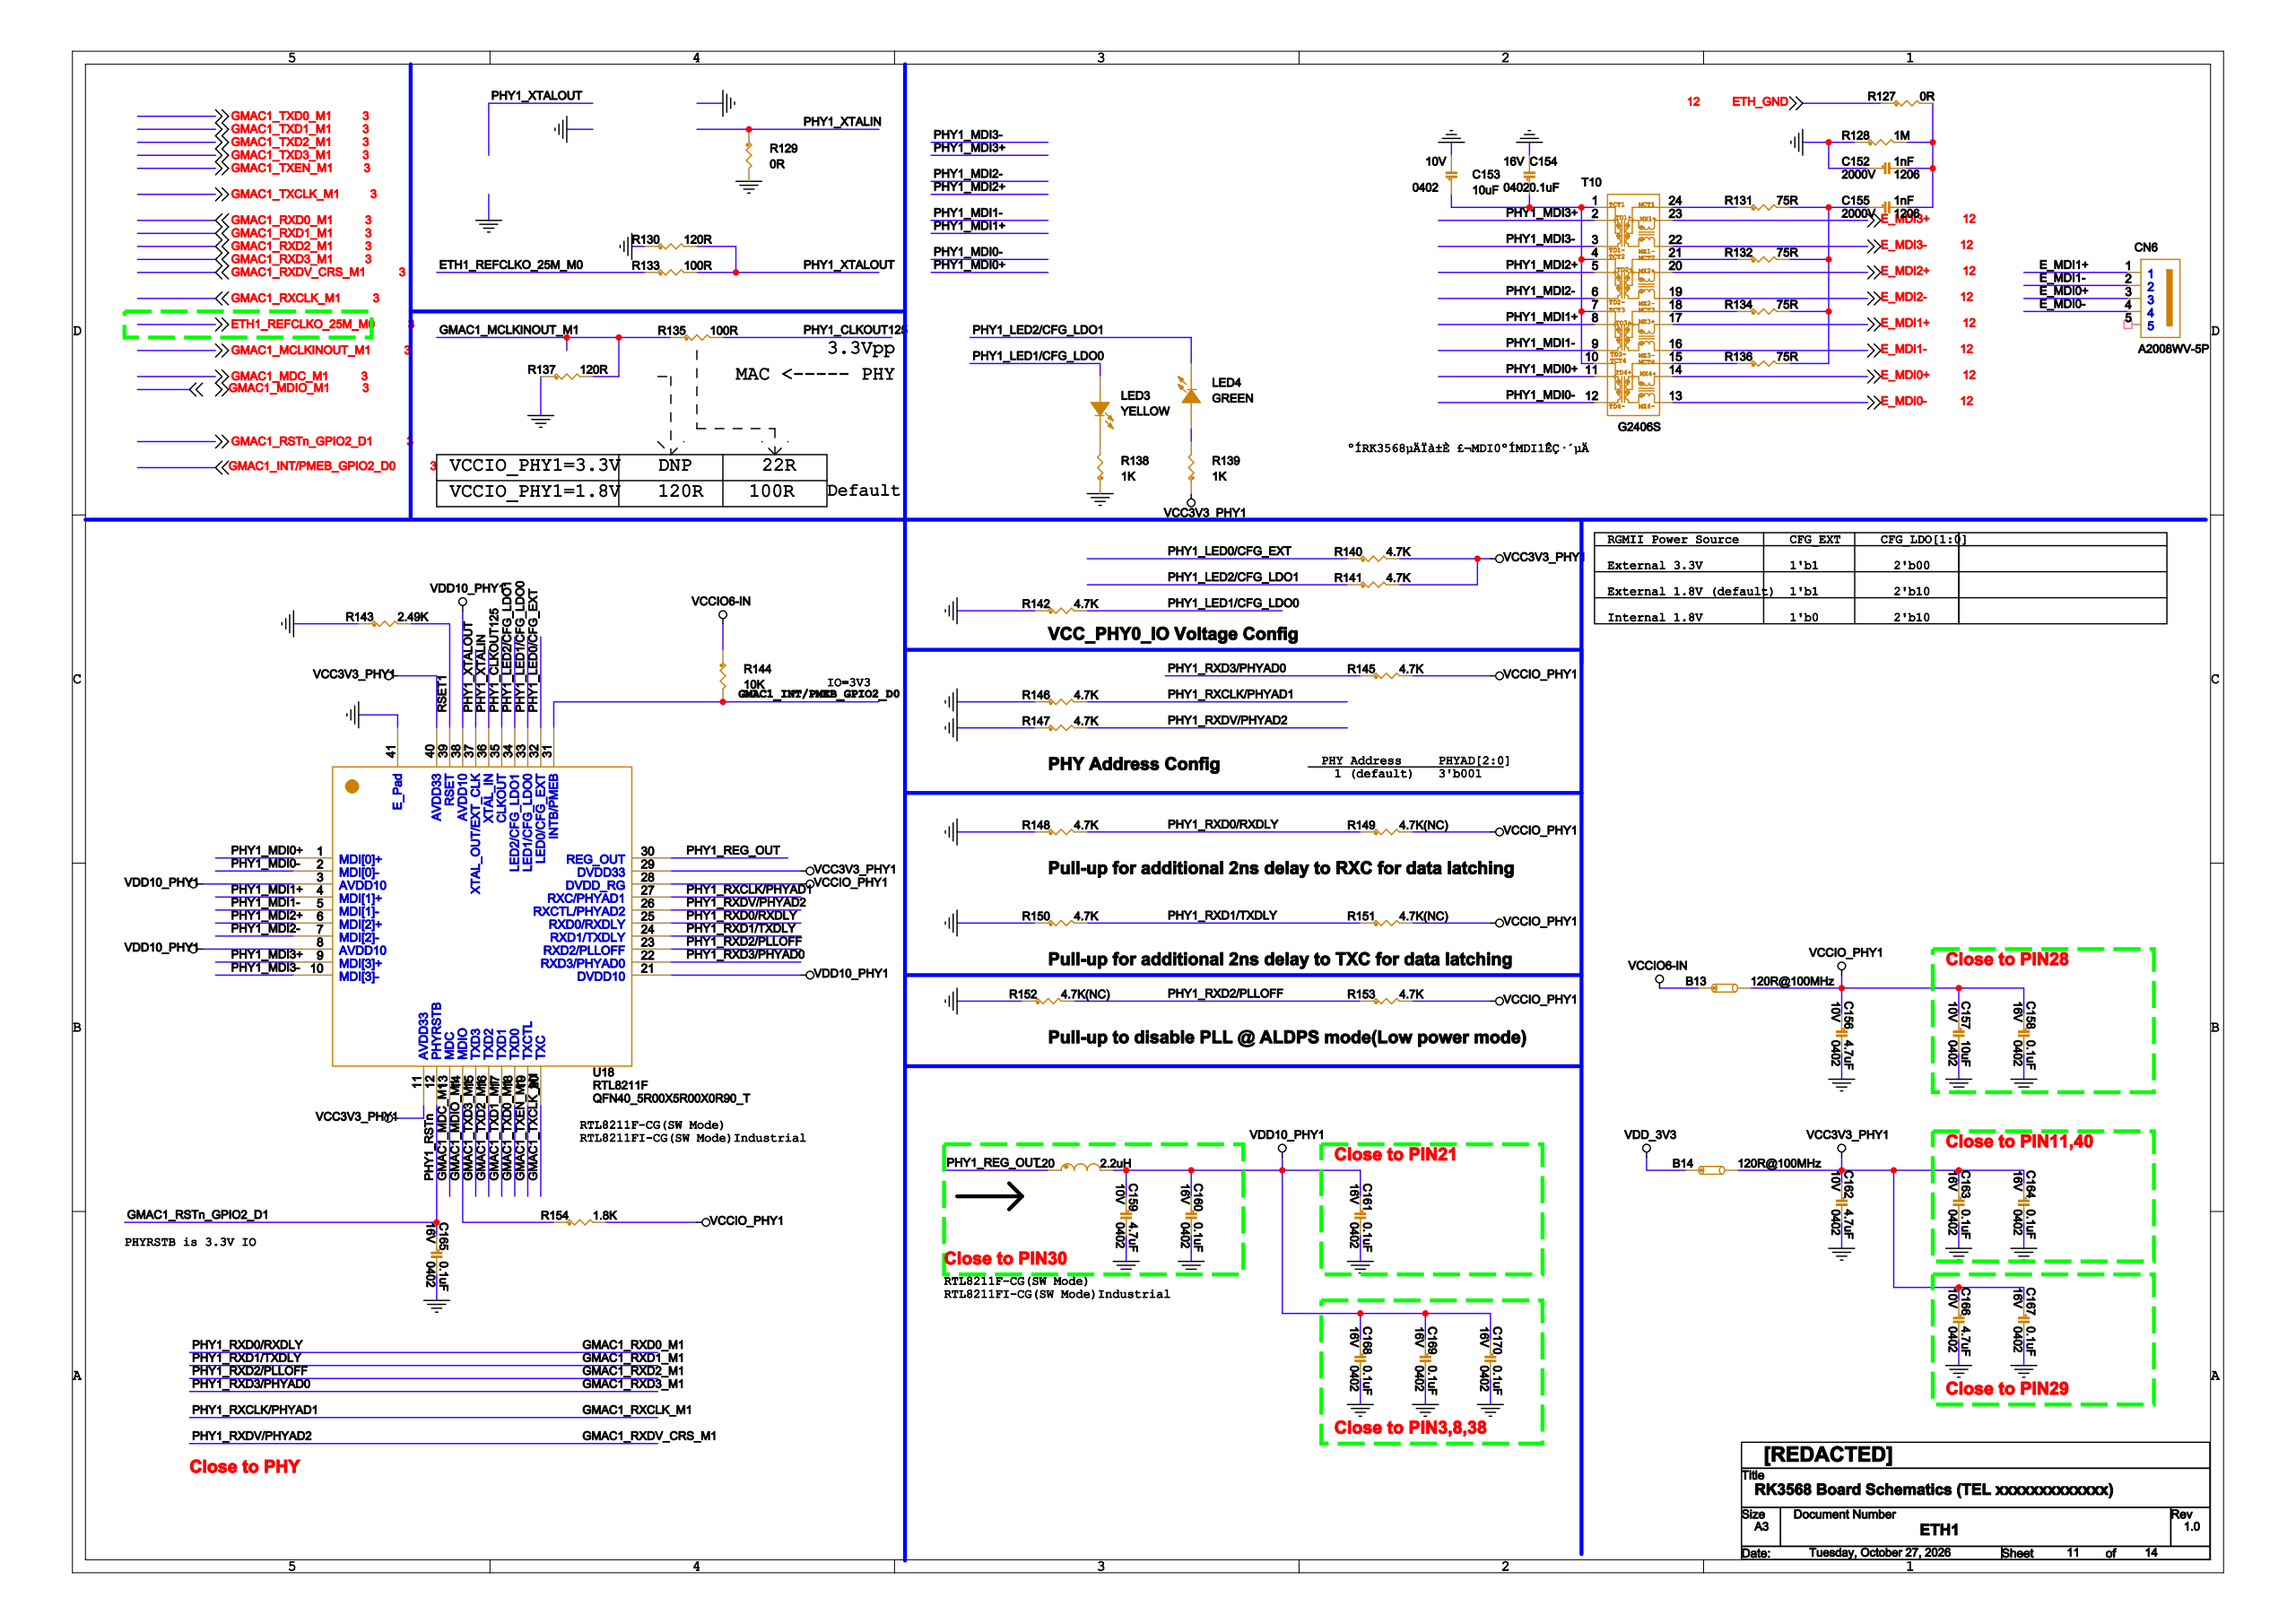Circuit board | Cadence Allegro | 669 parts | 581 nets | one sheet of the schematic
Parts on this sheet (reference | value | footprint):
B13 | 120R@100MHz | R0402
B14 | 120R@100MHz | R0402
C152 | 1nF | C1206
C153 | 10uF | C0402
C154 | 0.1uF | C0402
C155 | 1nF | C1206
C156 | 4.7uF | C0402
C157 | 10uF | C0402
C158 | 0.1uF | C0402
C159 | 4.7uF | C0402
C160 | 0.1uF | C0402
C161 | 0.1uF | C0402
C162 | 4.7uF | C0402
C163 | 0.1uF | C0402
C164 | 0.1uF | C0402
C165 | 0.1uF | C0402
C166 | 4.7uF | C0402
C167 | 0.1uF | C0402
C168 | 0.1uF | C0402
C169 | 0.1uF | C0402
C170 | 0.1uF | C0402
CN6 | A2008WV-5P | A2008WV_5P
L20 | 2.2uH | L2520
LED3 | YELLOW | D0603
LED4 | GREEN | D0603
R127 | 0R | R0402
R128 | 1M | R1206
R129 | 0R | R0402
R130 | 120R | R0402
R131 | 75R | R0402
R132 | 75R | R0402
R133 | 100R | R0402
R134 | 75R | R0402
R135 | 100R | R0402
R136 | 75R | R0402
R137 | 120R | R0402
R138 | 1K | R0402
R139 | 1K | R0402
R140 | 4.7K | R0402
R141 | 4.7K | R0402
R142 | 4.7K | R0402
R143 | 2.49K | R0402
R144 | 10K | R0402
R145 | 4.7K | R0402
R146 | 4.7K | R0402
R147 | 4.7K | R0402
R148 | 4.7K | R0402
R149 | 4.7K(NC) | R0402
R150 | 4.7K | R0402
R151 | 4.7K(NC) | R0402
R152 | 4.7K(NC) | R0402
R153 | 4.7K | R0402
R154 | 1.8K | R0402
T10 | G2406S | G2406S
U18 | RTL8211F | QFN40_5R00X5R00X0R90_T
Nets of these parts (net: part-pin ...):
GND: C152-1 C153-2 C154-2 C156-2 C157-2 C158-2 C159-2 C160-2 C161-2 C162-2 C163-2 C164-2 C165-2 C166-2 C167-2 C168-2 C169-2 C170-2 R128-1 R129-2 R130-1 R137-1 R138-1 R142-1 R143-1 R146-1 R147-1 R148-1 R150-1 R152-1 U18-41
VCC3V3_SYS: B14-1
VCCIO6-IN: B13-1 R144-1
VCCIO_PHY1: B13-2 C156-1 C157-1 C158-1 R145-2 R149-2 R151-2 R153-2 R154-2 U18-28
VCC3V3_PHY1: B14-2 C162-1 C163-1 C164-1 C166-1 C167-1 R139-1 R140-2 R141-2 U18-11 U18-29 U18-40
VDD10_PHY1: C159-1 C160-1 C161-1 C168-1 C169-1 C170-1 L20-2 U18-3 U18-8 U18-21 U18-38
N84615627: C153-1 C154-1 T10-1 T10-4 T10-7 T10-10
GMAC1_RSTN_GPIO2_D1: C165-1 U18-12
N84615441: C152-2 C155-2 R127-2 R128-2
N84615515: C155-1 R131-2 R132-2 R134-2 R136-2
E_MDI1+: CN6-1 T10-17
E_MDI1-: CN6-2 T10-16
E_MDI0+: CN6-3 T10-14
E_MDI0-: CN6-4 T10-13
PHY1_REG_OUT: L20-1 U18-30
PHY1_LED1/CFG_LDO0: LED3-1 R142-2 U18-33
N846141941: LED3-2 R138-2
N84614232: LED4-1 R139-2
PHY1_LED2/CFG_LDO1: LED4-2 R141-1 U18-34
ETH_GND: R127-1
PHY1_XTALIN: R129-1 U18-36
GMAC1_INT/PMEB_GPIO2_D0: R144-2 U18-31
N84615513: R131-1 T10-24
N84615503: R132-1 T10-21
N84615501: R134-1 T10-18
N84615499: R136-1 T10-15
GMAC1_RXD0_M1: R148-2 R149-1 U18-25
GMAC1_RXD1_M1: R150-2 R151-1 U18-24
GMAC1_RXD2_M1: R152-2 R153-1 U18-23
PHY1_XTALOUT: R130-2 R133-2 U18-37
GMAC1_MCLKINOUT_M1: R135-1 R137-2
ETH1_REFCLKO_25M_M0: R133-1
PHY1_CLKOUT125: R135-2 U18-35
PHY1_LED0/CFG_EXT: R140-1 U18-32
GMAC1_RXD3_M1: R145-1 U18-22
GMAC1_RXCLK_M1: R146-2 U18-27
GMAC1_RXDV_CRS_M1: R147-2 U18-26
RSET1: R143-2 U18-39
GMAC1_MDIO_M1: R154-1 U18-14
E_MDI3+: T10-23
E_MDI3-: T10-22
E_MDI2+: T10-20
E_MDI2-: T10-19
PHY1_MDI3+: T10-2 U18-9
PHY1_MDI3-: T10-3 U18-10
PHY1_MDI2+: T10-5 U18-6
PHY1_MDI2-: T10-6 U18-7
PHY1_MDI1+: T10-8 U18-4
PHY1_MDI1-: T10-9 U18-5
PHY1_MDI0+: T10-11 U18-1
PHY1_MDI0-: T10-12 U18-2
GMAC1_MDC_M1: U18-13
GMAC1_TXCLK_M1: U18-20
GMAC1_TXEN_M1: U18-19
GMAC1_TXD0_M1: U18-18
GMAC1_TXD1_M1: U18-17
GMAC1_TXD2_M1: U18-16
GMAC1_TXD3_M1: U18-15